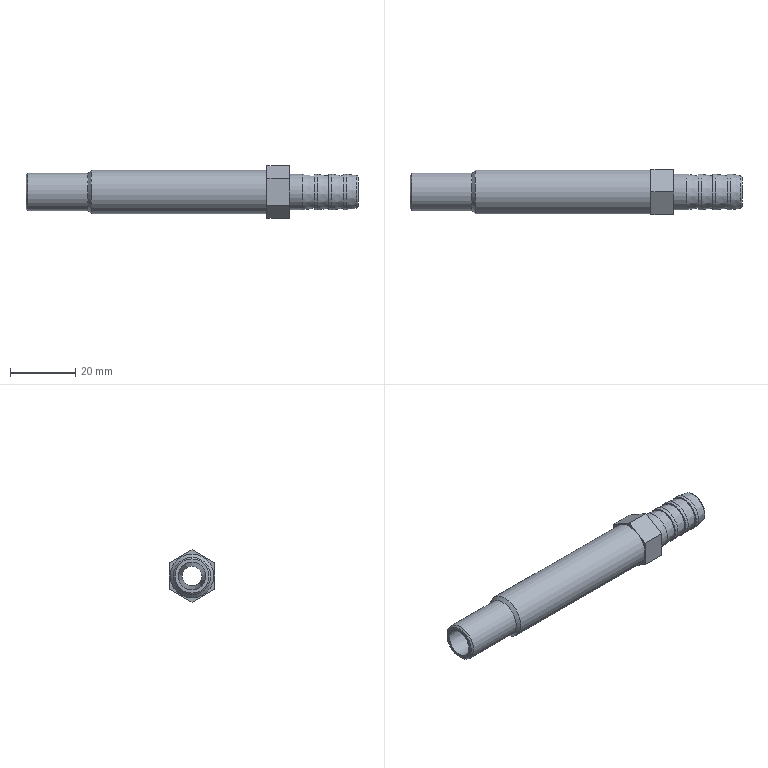Part | STEP file | solid 82 | 1 solid | 27 faces | box 102 x 14 x 16.166 mm | volume 8632 mm3 | plane 13 | cone 7 | cylinder 6 | torus 1 | commonest cylinder face diameters 11 x4 11.5 x1 13.5 x1